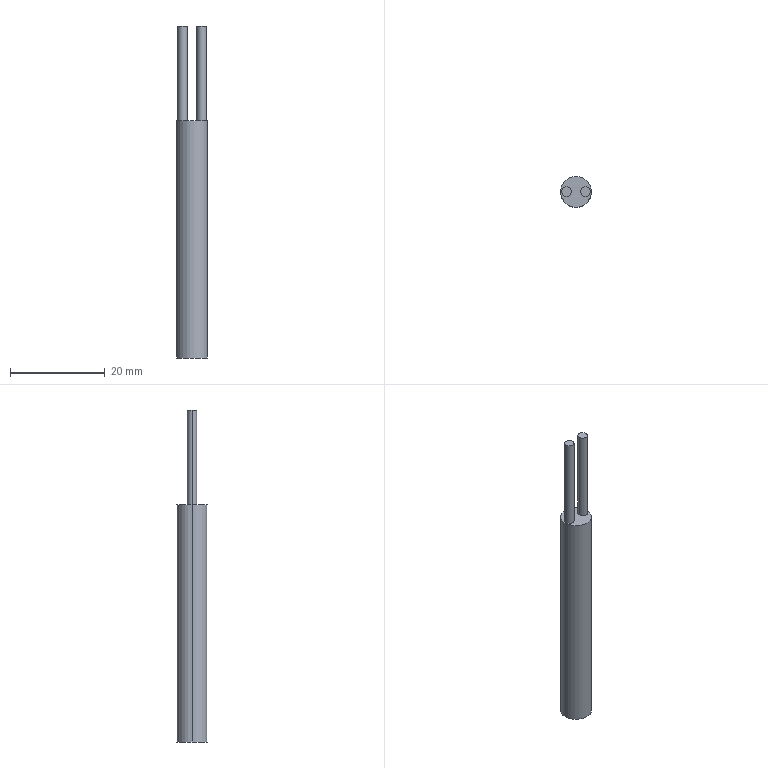Part | STEP file | 11-CC-MCH-6.5-50-100-100w-6-5011 | 1 solid | 10 faces | box 6.5 x 6.5 x 70 mm | volume 1785 mm3 | cylinder 6 | plane 4 | commonest cylinder face diameters 2 x4 6.5 x2
STEP:
#1=CARTESIAN_POINT('',(-298.821,207.256,-96.15));
#2=VERTEX_POINT('',#1);
#3=CARTESIAN_POINT('',(-296.821,207.256,-96.15));
#4=VERTEX_POINT('',#3);
#5=CARTESIAN_POINT('',(-297.821,207.256,-96.15));
#6=DIRECTION('',(0.,0.,1.));
#7=DIRECTION('',(1.,0.,0.));
#8=AXIS2_PLACEMENT_3D('',#5,#6,#7);
#9=CIRCLE('',#8,1.);
#10=EDGE_CURVE('',#2,#4,#9,.T.);
#11=ORIENTED_EDGE('',*,*,#10,.T.);
#12=CARTESIAN_POINT('',(-296.821,207.256,-76.15));
#13=VERTEX_POINT('',#12);
#14=CARTESIAN_POINT('',(-296.821,207.256,-96.15));
#15=DIRECTION('',(0.,0.,1.));
#16=VECTOR('',#15,1000.);
#17=LINE('',#14,#16);
#18=EDGE_CURVE('',#4,#13,#17,.T.);
#19=ORIENTED_EDGE('',*,*,#18,.T.);
#20=CARTESIAN_POINT('',(-298.821,207.256,-76.15));
#21=VERTEX_POINT('',#20);
#22=CARTESIAN_POINT('',(-297.821,207.256,-76.15));
#23=DIRECTION('',(0.,0.,-1.));
#24=DIRECTION('',(-1.,0.,0.));
#25=AXIS2_PLACEMENT_3D('',#22,#23,#24);
#26=CIRCLE('',#25,1.);
#27=EDGE_CURVE('',#13,#21,#26,.T.);
#28=ORIENTED_EDGE('',*,*,#27,.T.);
#29=CARTESIAN_POINT('',(-298.821,207.256,-96.15));
#30=DIRECTION('',(0.,0.,1.));
#31=VECTOR('',#30,1000.);
#32=LINE('',#29,#31);
#33=EDGE_CURVE('',#2,#21,#32,.T.);
#34=ORIENTED_EDGE('',*,*,#33,.F.);
#35=EDGE_LOOP('',(#11,#19,#28,#34));
#36=FACE_OUTER_BOUND('',#35,.T.);
#37=CARTESIAN_POINT('',(-297.821,207.256,-96.15));
#38=DIRECTION('',(0.,0.,1.));
#39=DIRECTION('',(-1.,0.,0.));
#40=AXIS2_PLACEMENT_3D('',#37,#38,#39);
#41=CYLINDRICAL_SURFACE('',#40,1.);
#42=ADVANCED_FACE('',(#36),#41,.T.);
#43=CARTESIAN_POINT('',(-292.821,207.256,-96.15));
#44=VERTEX_POINT('',#43);
#45=CARTESIAN_POINT('',(-294.821,207.256,-96.15));
#46=VERTEX_POINT('',#45);
#47=CARTESIAN_POINT('',(-293.821,207.256,-96.15));
#48=DIRECTION('',(0.,0.,1.));
#49=DIRECTION('',(1.,0.,0.));
#50=AXIS2_PLACEMENT_3D('',#47,#48,#49);
#51=CIRCLE('',#50,1.);
#52=EDGE_CURVE('',#44,#46,#51,.T.);
#53=ORIENTED_EDGE('',*,*,#52,.T.);
#54=CARTESIAN_POINT('',(-294.821,207.256,-76.15));
#55=VERTEX_POINT('',#54);
#56=CARTESIAN_POINT('',(-294.821,207.256,-96.15));
#57=DIRECTION('',(0.,0.,1.));
#58=VECTOR('',#57,1000.);
#59=LINE('',#56,#58);
#60=EDGE_CURVE('',#46,#55,#59,.T.);
#61=ORIENTED_EDGE('',*,*,#60,.T.);
#62=CARTESIAN_POINT('',(-292.821,207.256,-76.15));
#63=VERTEX_POINT('',#62);
#64=CARTESIAN_POINT('',(-293.821,207.256,-76.15));
#65=DIRECTION('',(0.,0.,1.));
#66=DIRECTION('',(1.,0.,0.));
#67=AXIS2_PLACEMENT_3D('',#64,#65,#66);
#68=CIRCLE('',#67,1.);
#69=EDGE_CURVE('',#63,#55,#68,.T.);
#70=ORIENTED_EDGE('',*,*,#69,.F.);
#71=CARTESIAN_POINT('',(-292.821,207.256,-96.15));
#72=DIRECTION('',(0.,0.,1.));
#73=VECTOR('',#72,1000.);
#74=LINE('',#71,#73);
#75=EDGE_CURVE('',#44,#63,#74,.T.);
#76=ORIENTED_EDGE('',*,*,#75,.F.);
#77=EDGE_LOOP('',(#53,#61,#70,#76));
#78=FACE_OUTER_BOUND('',#77,.T.);
#79=CARTESIAN_POINT('',(-293.821,207.256,-96.15));
#80=DIRECTION('',(0.,0.,1.));
#81=DIRECTION('',(1.,0.,0.));
#82=AXIS2_PLACEMENT_3D('',#79,#80,#81);
#83=CYLINDRICAL_SURFACE('',#82,1.);
#84=ADVANCED_FACE('',(#78),#83,.T.);
#85=CARTESIAN_POINT('',(-292.571,207.256,-96.15));
#86=VERTEX_POINT('',#85);
#87=CARTESIAN_POINT('',(-299.071,207.256,-96.15));
#88=VERTEX_POINT('',#87);
#89=CARTESIAN_POINT('',(-295.821,207.256,-96.15));
#90=DIRECTION('',(0.,0.,1.));
#91=DIRECTION('',(1.,0.,0.));
#92=AXIS2_PLACEMENT_3D('',#89,#90,#91);
#93=CIRCLE('',#92,3.25);
#94=EDGE_CURVE('',#86,#88,#93,.T.);
#95=ORIENTED_EDGE('',*,*,#94,.F.);
#96=CARTESIAN_POINT('',(-292.571,207.256,-146.15));
#97=VERTEX_POINT('',#96);
#98=CARTESIAN_POINT('',(-292.571,207.256,-96.15));
#99=DIRECTION('',(0.,0.,-1.));
#100=VECTOR('',#99,1000.);
#101=LINE('',#98,#100);
#102=EDGE_CURVE('',#86,#97,#101,.T.);
#103=ORIENTED_EDGE('',*,*,#102,.T.);
#104=CARTESIAN_POINT('',(-299.071,207.256,-146.15));
#105=VERTEX_POINT('',#104);
#106=CARTESIAN_POINT('',(-295.821,207.256,-146.15));
#107=DIRECTION('',(0.,0.,1.));
#108=DIRECTION('',(1.,0.,0.));
#109=AXIS2_PLACEMENT_3D('',#106,#107,#108);
#110=CIRCLE('',#109,3.25);
#111=EDGE_CURVE('',#97,#105,#110,.T.);
#112=ORIENTED_EDGE('',*,*,#111,.T.);
#113=CARTESIAN_POINT('',(-299.071,207.256,-96.15));
#114=DIRECTION('',(0.,0.,-1.));
#115=VECTOR('',#114,1000.);
#116=LINE('',#113,#115);
#117=EDGE_CURVE('',#88,#105,#116,.T.);
#118=ORIENTED_EDGE('',*,*,#117,.F.);
#119=EDGE_LOOP('',(#95,#103,#112,#118));
#120=FACE_OUTER_BOUND('',#119,.T.);
#121=CARTESIAN_POINT('',(-295.821,207.256,-96.15));
#122=DIRECTION('',(0.,0.,-1.));
#123=DIRECTION('',(-1.,0.,0.));
#124=AXIS2_PLACEMENT_3D('',#121,#122,#123);
#125=CYLINDRICAL_SURFACE('',#124,3.25);
#126=ADVANCED_FACE('',(#120),#125,.T.);
#127=ORIENTED_EDGE('',*,*,#102,.F.);
#128=CARTESIAN_POINT('',(-295.821,207.256,-96.15));
#129=DIRECTION('',(0.,0.,1.));
#130=DIRECTION('',(1.,0.,0.));
#131=AXIS2_PLACEMENT_3D('',#128,#129,#130);
#132=CIRCLE('',#131,3.25);
#133=EDGE_CURVE('',#88,#86,#132,.T.);
#134=ORIENTED_EDGE('',*,*,#133,.F.);
#135=ORIENTED_EDGE('',*,*,#117,.T.);
#136=CARTESIAN_POINT('',(-295.821,207.256,-146.15));
#137=DIRECTION('',(0.,0.,1.));
#138=DIRECTION('',(1.,0.,0.));
#139=AXIS2_PLACEMENT_3D('',#136,#137,#138);
#140=CIRCLE('',#139,3.25);
#141=EDGE_CURVE('',#105,#97,#140,.T.);
#142=ORIENTED_EDGE('',*,*,#141,.T.);
#143=EDGE_LOOP('',(#127,#134,#135,#142));
#144=FACE_OUTER_BOUND('',#143,.T.);
#145=CARTESIAN_POINT('',(-295.821,207.256,-96.15));
#146=DIRECTION('',(0.,0.,-1.));
#147=DIRECTION('',(-1.,0.,0.));
#148=AXIS2_PLACEMENT_3D('',#145,#146,#147);
#149=CYLINDRICAL_SURFACE('',#148,3.25);
#150=ADVANCED_FACE('',(#144),#149,.T.);
#151=ORIENTED_EDGE('',*,*,#10,.F.);
#152=CARTESIAN_POINT('',(-297.821,207.256,-96.15));
#153=DIRECTION('',(0.,0.,1.));
#154=DIRECTION('',(1.,0.,0.));
#155=AXIS2_PLACEMENT_3D('',#152,#153,#154);
#156=CIRCLE('',#155,1.);
#157=EDGE_CURVE('',#4,#2,#156,.T.);
#158=ORIENTED_EDGE('',*,*,#157,.F.);
#159=EDGE_LOOP('',(#151,#158));
#160=FACE_BOUND('',#159,.T.);
#161=ORIENTED_EDGE('',*,*,#52,.F.);
#162=CARTESIAN_POINT('',(-293.821,207.256,-96.15));
#163=DIRECTION('',(0.,0.,1.));
#164=DIRECTION('',(1.,0.,0.));
#165=AXIS2_PLACEMENT_3D('',#162,#163,#164);
#166=CIRCLE('',#165,1.);
#167=EDGE_CURVE('',#46,#44,#166,.T.);
#168=ORIENTED_EDGE('',*,*,#167,.F.);
#169=EDGE_LOOP('',(#161,#168));
#170=FACE_BOUND('',#169,.T.);
#171=ORIENTED_EDGE('',*,*,#133,.T.);
#172=ORIENTED_EDGE('',*,*,#94,.T.);
#173=EDGE_LOOP('',(#171,#172));
#174=FACE_OUTER_BOUND('',#173,.T.);
#175=CARTESIAN_POINT('',(-295.821,207.256,-96.15));
#176=DIRECTION('',(0.,0.,1.));
#177=DIRECTION('',(1.,0.,0.));
#178=AXIS2_PLACEMENT_3D('',#175,#176,#177);
#179=PLANE('',#178);
#180=ADVANCED_FACE('',(#160,#170,#174),#179,.T.);
#181=ORIENTED_EDGE('',*,*,#141,.F.);
#182=ORIENTED_EDGE('',*,*,#111,.F.);
#183=EDGE_LOOP('',(#181,#182));
#184=FACE_OUTER_BOUND('',#183,.T.);
#185=CARTESIAN_POINT('',(-295.821,207.256,-146.15));
#186=DIRECTION('',(0.,0.,1.));
#187=DIRECTION('',(1.,0.,0.));
#188=AXIS2_PLACEMENT_3D('',#185,#186,#187);
#189=PLANE('',#188);
#190=ADVANCED_FACE('',(#184),#189,.F.);
#191=ORIENTED_EDGE('',*,*,#69,.T.);
#192=CARTESIAN_POINT('',(-293.821,207.256,-76.15));
#193=DIRECTION('',(0.,0.,1.));
#194=DIRECTION('',(1.,0.,0.));
#195=AXIS2_PLACEMENT_3D('',#192,#193,#194);
#196=CIRCLE('',#195,1.);
#197=EDGE_CURVE('',#55,#63,#196,.T.);
#198=ORIENTED_EDGE('',*,*,#197,.T.);
#199=EDGE_LOOP('',(#191,#198));
#200=FACE_OUTER_BOUND('',#199,.T.);
#201=CARTESIAN_POINT('',(-293.821,207.256,-76.15));
#202=DIRECTION('',(0.,0.,1.));
#203=DIRECTION('',(1.,0.,0.));
#204=AXIS2_PLACEMENT_3D('',#201,#202,#203);
#205=PLANE('',#204);
#206=ADVANCED_FACE('',(#200),#205,.T.);
#207=ORIENTED_EDGE('',*,*,#60,.F.);
#208=ORIENTED_EDGE('',*,*,#167,.T.);
#209=ORIENTED_EDGE('',*,*,#75,.T.);
#210=ORIENTED_EDGE('',*,*,#197,.F.);
#211=EDGE_LOOP('',(#207,#208,#209,#210));
#212=FACE_OUTER_BOUND('',#211,.T.);
#213=CARTESIAN_POINT('',(-293.821,207.256,-96.15));
#214=DIRECTION('',(0.,0.,1.));
#215=DIRECTION('',(1.,0.,0.));
#216=AXIS2_PLACEMENT_3D('',#213,#214,#215);
#217=CYLINDRICAL_SURFACE('',#216,1.);
#218=ADVANCED_FACE('',(#212),#217,.T.);
#219=CARTESIAN_POINT('',(-297.821,207.256,-76.15));
#220=DIRECTION('',(0.,0.,-1.));
#221=DIRECTION('',(-1.,0.,0.));
#222=AXIS2_PLACEMENT_3D('',#219,#220,#221);
#223=CIRCLE('',#222,1.);
#224=EDGE_CURVE('',#21,#13,#223,.T.);
#225=ORIENTED_EDGE('',*,*,#224,.F.);
#226=ORIENTED_EDGE('',*,*,#27,.F.);
#227=EDGE_LOOP('',(#225,#226));
#228=FACE_OUTER_BOUND('',#227,.T.);
#229=CARTESIAN_POINT('',(-297.821,207.256,-76.15));
#230=DIRECTION('',(0.,0.,1.));
#231=DIRECTION('',(-1.,0.,0.));
#232=AXIS2_PLACEMENT_3D('',#229,#230,#231);
#233=PLANE('',#232);
#234=ADVANCED_FACE('',(#228),#233,.T.);
#235=ORIENTED_EDGE('',*,*,#18,.F.);
#236=ORIENTED_EDGE('',*,*,#157,.T.);
#237=ORIENTED_EDGE('',*,*,#33,.T.);
#238=ORIENTED_EDGE('',*,*,#224,.T.);
#239=EDGE_LOOP('',(#235,#236,#237,#238));
#240=FACE_OUTER_BOUND('',#239,.T.);
#241=CARTESIAN_POINT('',(-297.821,207.256,-96.15));
#242=DIRECTION('',(0.,0.,1.));
#243=DIRECTION('',(-1.,0.,0.));
#244=AXIS2_PLACEMENT_3D('',#241,#242,#243);
#245=CYLINDRICAL_SURFACE('',#244,1.);
#246=ADVANCED_FACE('',(#240),#245,.T.);
#247=CLOSED_SHELL('',(#42,#84,#126,#150,#180,#190,#206,#218,#234,#246));
#248=MANIFOLD_SOLID_BREP('',#247);
#249=CARTESIAN_POINT('',(0.,0.,0.));
#250=DIRECTION('',(0.,0.,1.));
#251=DIRECTION('',(1.,0.,0.));
#252=AXIS2_PLACEMENT_3D('',#249,#250,#251);
#253=(LENGTH_UNIT()NAMED_UNIT(*)SI_UNIT(.MILLI.,.METRE.));
#254=UNCERTAINTY_MEASURE_WITH_UNIT(LENGTH_MEASURE(0.00001),#253,'','');
#255=(NAMED_UNIT(*)PLANE_ANGLE_UNIT()SI_UNIT($,.RADIAN.));
#256=(NAMED_UNIT(*)SI_UNIT($,.STERADIAN.)SOLID_ANGLE_UNIT());
#257=(GEOMETRIC_REPRESENTATION_CONTEXT(3)GLOBAL_UNCERTAINTY_ASSIGNED_CONTEXT((#254))GLOBAL_UNIT_ASSIGNED_CONTEXT((#253,#255,#256))REPRESENTATION_CONTEXT('',''));
#258=ADVANCED_BREP_SHAPE_REPRESENTATION('',(#248,#252),#257);